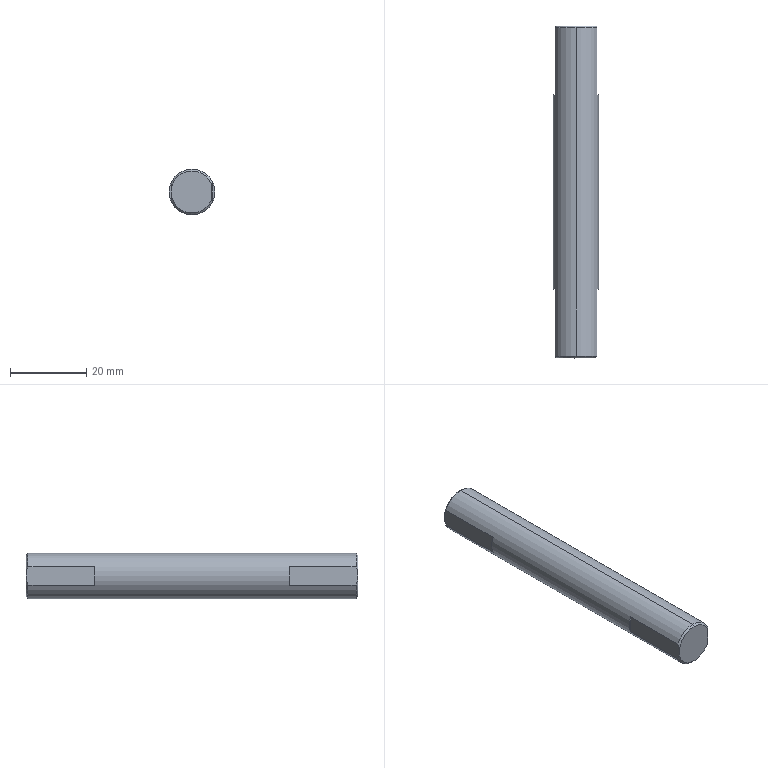Part | STEP file | ND25021-01-JDKM-09-GJ | 1 solid | 19 faces | box 12 x 87 x 12 mm | volume 9716 mm3 | plane 11 | cone 6 | cylinder 2 | commonest cylinder face diameters 12 x2